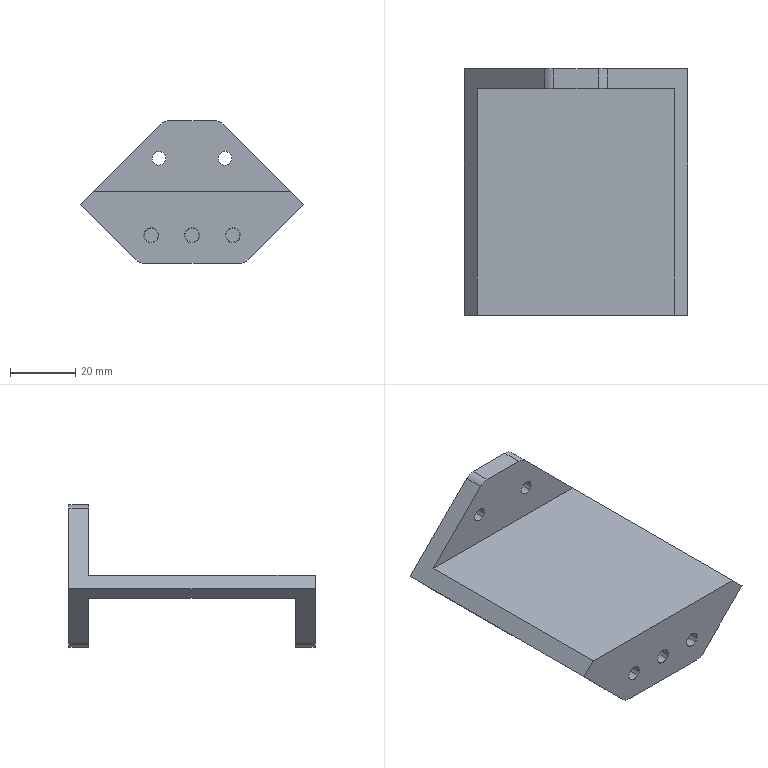NC program | NX | posted with a generic post | part box 68.307 x 75.3 x 43.668 mm
Whole program:
N10 G17 G21 G94 G90
(DRILLING_COPY_1_COPY , TOOL : D6A45)
N12 T01 M6
N14 G54
N16 G17 G0 G90 X-10.111 Y10.309 B0. C0. S5000 M3
N18 G43 Z30. H1
N20 G94 G81 G98 Z-1. F350. R3.
N22 X10.111
N24 X-4.95 Y15.47
N26 X4.243 Y6.278
N28 G80
N30 G0 X4.243 Y6.278 Z30.
N32 M5
(DRILLING_COPY_1_COPY_1_1_COPY_1 , TOOL : 4.2ZT)
N34 T04 M6
N36 G54
N38 G17 G0 G90 X-10.111 Y10.309 B0. C0. S2000 M3
N40 G43 Z30. H4
N42 G94 G83 G98 Z-8.762 F200. Q2. R3.
N44 X10.111
N46 G80
N48 G0 X10.111 Y10.309 Z30.
N50 M5
(HOLE_MILLING , TOOL : D3)
N52 T03 M6
N54 G54
N56 G17 G0 G90 X-4.95 Y15.47 B0. C0. S9500 M3
N58 G43 Z30. H3
N60 Z0.5
N62 G94 G3 X-5.15 Y15.67 R0.2 F1250.
N64 X-5.35 Y15.47 R0.2
N66 X-5.35 Y15.47 Z0.3 I0.4 J0.
N68 X-5.35 Y15.47 Z0.1 I0.4 J0.
N70 X-5.35 Y15.47 Z-0.1 I0.4 J0.
N72 X-5.35 Y15.47 Z-0.3 I0.4 J0.
N74 X-5.35 Y15.47 Z-0.5 I0.4 J0.
N76 X-5.35 Y15.47 Z-0.7 I0.4 J0.
N78 X-5.35 Y15.47 Z-0.9 I0.4 J0.
N80 X-5.35 Y15.47 Z-1.1 I0.4 J0.
N82 X-5.35 Y15.47 Z-1.3 I0.4 J0.
N84 X-5.35 Y15.47 Z-1.5 I0.4 J0.
N86 X-5.35 Y15.47 Z-1.7 I0.4 J0.
N88 X-5.35 Y15.47 Z-1.9 I0.4 J0.
N90 X-5.35 Y15.47 Z-2.1 I0.4 J0.
N92 X-5.35 Y15.47 Z-2.3 I0.4 J0.
N94 X-5.35 Y15.47 Z-2.5 I0.4 J0.
N96 X-5.35 Y15.47 Z-2.7 I0.4 J0.
N98 X-5.35 Y15.47 Z-2.9 I0.4 J0.
N100 X-5.35 Y15.47 Z-3.1 I0.4 J0.
N102 X-5.35 Y15.47 Z-3.3 I0.4 J0.
N104 X-5.35 Y15.47 Z-3.5 I0.4 J0.
N106 X-5.35 Y15.47 Z-3.7 I0.4 J0.
N108 X-5.35 Y15.47 Z-3.9 I0.4 J0.
N110 X-4.55 Y15.47 Z-4. I0.4 J0.
N112 X-4.95 Y15.87 R0.4
N114 X-4.55 Y15.47 R-0.4
N116 X-4.75 Y15.67 R0.2
N118 X-4.95 Y15.47 R0.2
N120 G0 Z30.
N122 X4.243 Y6.278
N124 Z0.5
N126 G3 X4.043 Y6.478 R0.2
N128 X3.843 Y6.278 R0.2
N130 X3.843 Y6.278 Z0.3 I0.4 J0.
N132 X3.843 Y6.278 Z0.1 I0.4 J0.
N134 X3.843 Y6.278 Z-0.1 I0.4 J0.
N136 X3.843 Y6.278 Z-0.3 I0.4 J0.
N138 X3.843 Y6.278 Z-0.5 I0.4 J0.
N140 X3.843 Y6.278 Z-0.7 I0.4 J0.
N142 X3.843 Y6.278 Z-0.9 I0.4 J0.
N144 X3.843 Y6.278 Z-1.1 I0.4 J0.
N146 X3.843 Y6.278 Z-1.3 I0.4 J0.
N148 X3.843 Y6.278 Z-1.5 I0.4 J0.
N150 X3.843 Y6.278 Z-1.7 I0.4 J0.
N152 X3.843 Y6.278 Z-1.9 I0.4 J0.
N154 X3.843 Y6.278 Z-2.1 I0.4 J0.
N156 X3.843 Y6.278 Z-2.3 I0.4 J0.
N158 X3.843 Y6.278 Z-2.5 I0.4 J0.
N160 X3.843 Y6.278 Z-2.7 I0.4 J0.
N162 X3.843 Y6.278 Z-2.9 I0.4 J0.
N164 X3.843 Y6.278 Z-3.1 I0.4 J0.
N166 X3.843 Y6.278 Z-3.3 I0.4 J0.
N168 X3.843 Y6.278 Z-3.5 I0.4 J0.
N170 X3.843 Y6.278 Z-3.7 I0.4 J0.
N172 X3.843 Y6.278 Z-3.9 I0.4 J0.
N174 X4.643 Y6.278 Z-4. I0.4 J0.
N176 X4.243 Y6.678 R0.4
N178 X4.643 Y6.278 R-0.4
N180 X4.443 Y6.478 R0.2
N182 X4.243 Y6.278 R0.2
N184 G0 Z30.
N186 M5
(PLANAR_MILL_COPY_COPY_COPY_COPY_COPY_COPY_1_COPY_1_COPY_1_1 , TOOL : D6A45)
N188 T01 M6
N190 G54
N192 G17 G0 G90 X-10.038 Y10.376 B0. C0. S9500 M3
N194 G43 Z30. H1
N196 Z0.5
N198 G94 G1 Z-1. F1250.
N200 X-9.245 Y11.109
N202 G3 X-10.111 Y11.609 R1.
N204 X-11.411 Y10.309 R1.3
N206 X-10.111 Y11.609 R-1.3
N208 X-10.977 Y11.109 R1.
N210 G1 X-10.185 Y10.376
N212 Z0.5
N214 G0 Z30.
N216 X-6.142 Y15.341
N218 Z0.5
N220 G1 X-5.989 Y14.812 Z0.353
N222 X-5.607 Y14.431 Z0.208
N224 X-4.95 Y14.24 Z0.025
N226 X-4.292 Y14.431 Z-0.159
N228 X-3.91 Y14.812 Z-0.304
N230 X-3.72 Y15.47 Z-0.487
N232 X-3.91 Y16.128 Z-0.671
N234 X-4.292 Y16.509 Z-0.815
N236 X-4.68 Y16.67 Z-0.928
N238 X-4.95 Z-1.
N240 G3 X-6.15 Y15.47 R1.2
N242 X-4.95 Y16.67 R-1.2
N244 X-5.816 Y16.17 R1.
N246 G1 Z0.5
N248 G0 Z30.
N250 X3.05 Y6.148
N252 Z0.5
N254 G1 X3.203 Y5.62 Z0.353
N256 X3.585 Y5.238 Z0.208
N258 X4.243 Y5.048 Z0.025
N260 X4.9 Y5.238 Z-0.159
N262 X5.282 Y5.62 Z-0.304
N264 X5.473 Y6.278 Z-0.487
N266 X5.282 Y6.935 Z-0.671
N268 X4.9 Y7.317 Z-0.815
N270 X4.513 Y7.478 Z-0.928
N272 X4.243 Z-1.
N274 G3 X3.043 Y6.278 R1.2
N276 X4.243 Y7.478 R-1.2
N278 X3.377 Y6.978 R1.
N280 G1 Z0.5
N282 G0 Z30.
N284 X10.185 Y10.376
N286 Z0.5
N288 G1 Z-1.
N290 X10.977 Y11.109
N292 G3 X10.111 Y11.609 R1.
N294 X8.811 Y10.309 R1.3
N296 X10.111 Y11.609 R-1.3
N298 X9.245 Y11.109 R1.
N300 G1 X10.038 Y10.376
N302 Z0.5
N304 G0 Z30.
N306 M5
(CUTTERCOMP3 , TOOL : D3)
N308 T03 M6
N310 G54
N312 G17 G0 G90 X-4.95 Y15.47 B0. C0. S9500 M3
N314 G43 Z30. H3
N316 Z0.5
N318 G41 G94 G1 X-4.977 Y15.566 F1000. D3
N320 G3 X-5.4 Y15.47 R0.222
N322 X-5.4 Y15.47 Z-0.5 I0.45 J0.
N324 X-5.4 Y15.47 Z-1.5 I0.45 J0.
N326 X-5.4 Y15.47 Z-2.5 I0.45 J0.
N328 X-5.4 Y15.47 Z-3.5 I0.45 J0.
N330 X-4.5 Y15.47 Z-4. I0.45 J0.
N332 X-4.95 Y15.92 R0.45
N334 X-4.5 Y15.47 R-0.45
N336 X-4.923 Y15.566 R0.222
N338 G40
N340 G1 X-4.95 Y15.47
N342 G0 Z30.
N344 X4.243 Y6.278
N346 Z0.5
N348 G41 G1 X4.216 Y6.374
N350 G3 X3.793 Y6.278 R0.222
N352 X3.793 Y6.278 Z-0.5 I0.45 J0.
N354 X3.793 Y6.278 Z-1.5 I0.45 J0.
N356 X3.793 Y6.278 Z-2.5 I0.45 J0.
N358 X3.793 Y6.278 Z-3.5 I0.45 J0.
N360 X4.693 Y6.278 Z-4. I0.45 J0.
N362 X4.243 Y6.728 R0.45
N364 X4.693 Y6.278 R-0.45
N366 X4.27 Y6.374 R0.222
N368 G40
N370 G1 X4.243 Y6.278
N372 G0 Z30.
N374 M5
N376 M2